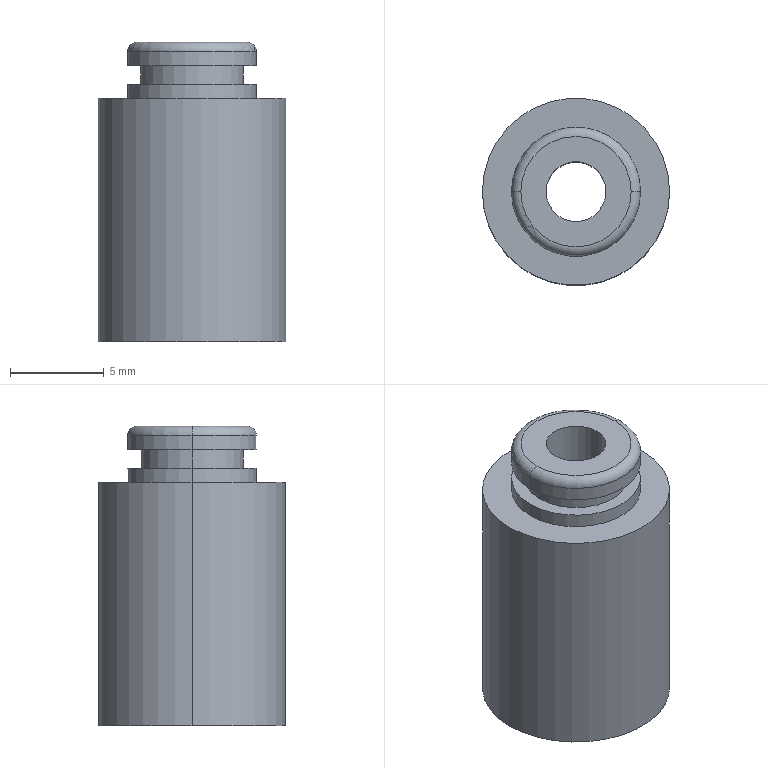Part | STEP file | SS5V1-16S3AD-08B-N1_VV5Q Fittings | 1 solid | 17 faces | box 10 x 10 x 16 mm | volume 989.757 mm3 | cylinder 10 | plane 5 | torus 2 | commonest cylinder face diameters 6.9 x4 3.2 x2 5.5 x2 10 x2
STEP:
#1=CARTESIAN_POINT('',(0.,0.,0.));
#2=DIRECTION('',(0.,0.,1.));
#3=DIRECTION('',(1.,0.,0.));
#4=AXIS2_PLACEMENT_3D('',#1,#2,#3);
#5=CARTESIAN_POINT('',(-3.45,0.,15.5));
#6=VERTEX_POINT('',#5);
#7=CARTESIAN_POINT('',(3.45,0.,15.5));
#8=VERTEX_POINT('',#7);
#9=CARTESIAN_POINT('',(0.,0.,15.5));
#10=DIRECTION('',(0.,0.,-1.));
#11=DIRECTION('',(1.,0.,0.));
#12=AXIS2_PLACEMENT_3D('',#9,#10,#11);
#13=CIRCLE('',#12,3.45);
#14=CARTESIAN_POINT('',(0.,0.,15.5));
#15=DIRECTION('',(0.,0.,1.));
#16=DIRECTION('',(1.,0.,0.));
#17=AXIS2_PLACEMENT_3D('',#14,#15,#16);
#18=TOROIDAL_SURFACE('',#17,2.95,0.5);
#19=CARTESIAN_POINT('',(6.283,0.));
#20=DIRECTION('',(-1.,0.));
#21=VECTOR('',#20,1.);
#22=LINE('',#19,#21);
#23=(GEOMETRIC_REPRESENTATION_CONTEXT(2)PARAMETRIC_REPRESENTATION_CONTEXT()REPRESENTATION_CONTEXT('',''));
#24=DEFINITIONAL_REPRESENTATION('',(#22),#23);
#25=PCURVE('',#18,#24);
#26=CARTESIAN_POINT('',(0.,0.,16.));
#27=DIRECTION('',(0.,0.,-1.));
#28=DIRECTION('',(-1.,0.,0.));
#29=AXIS2_PLACEMENT_3D('',#26,#27,#28);
#30=CYLINDRICAL_SURFACE('',#29,3.45);
#31=CARTESIAN_POINT('',(-3.142,0.5));
#32=DIRECTION('',(1.,0.));
#33=VECTOR('',#32,1.);
#34=LINE('',#31,#33);
#35=(GEOMETRIC_REPRESENTATION_CONTEXT(2)PARAMETRIC_REPRESENTATION_CONTEXT()REPRESENTATION_CONTEXT('',''));
#36=DEFINITIONAL_REPRESENTATION('',(#34),#35);
#37=PCURVE('',#30,#36);
#38=SURFACE_CURVE('',#13,(#25,#37),.PCURVE_S1.);
#39=EDGE_CURVE('',#6,#8,#38,.T.);
#40=ORIENTED_EDGE('',*,*,#39,.F.);
#41=CARTESIAN_POINT('',(-2.95,0.,16.));
#42=VERTEX_POINT('',#41);
#43=CARTESIAN_POINT('',(-2.95,0.,15.5));
#44=DIRECTION('',(0.,1.,0.));
#45=DIRECTION('',(-1.,0.,0.));
#46=AXIS2_PLACEMENT_3D('',#43,#44,#45);
#47=CIRCLE('',#46,0.5);
#48=CARTESIAN_POINT('',(3.142,0.));
#49=DIRECTION('',(0.,1.));
#50=VECTOR('',#49,1.);
#51=LINE('',#48,#50);
#52=(GEOMETRIC_REPRESENTATION_CONTEXT(2)PARAMETRIC_REPRESENTATION_CONTEXT()REPRESENTATION_CONTEXT('',''));
#53=DEFINITIONAL_REPRESENTATION('',(#51),#52);
#54=PCURVE('',#18,#53);
#55=CARTESIAN_POINT('',(0.,0.,15.5));
#56=DIRECTION('',(0.,0.,1.));
#57=DIRECTION('',(1.,0.,0.));
#58=AXIS2_PLACEMENT_3D('',#55,#56,#57);
#59=TOROIDAL_SURFACE('',#58,2.95,0.5);
#60=CARTESIAN_POINT('',(3.142,0.));
#61=DIRECTION('',(0.,1.));
#62=VECTOR('',#61,1.);
#63=LINE('',#60,#62);
#64=(GEOMETRIC_REPRESENTATION_CONTEXT(2)PARAMETRIC_REPRESENTATION_CONTEXT()REPRESENTATION_CONTEXT('',''));
#65=DEFINITIONAL_REPRESENTATION('',(#63),#64);
#66=PCURVE('',#59,#65);
#67=SURFACE_CURVE('',#47,(#54,#66),.PCURVE_S1.);
#68=EDGE_CURVE('',#6,#42,#67,.T.);
#69=ORIENTED_EDGE('',*,*,#68,.T.);
#70=CARTESIAN_POINT('',(2.95,0.,16.));
#71=VERTEX_POINT('',#70);
#72=CARTESIAN_POINT('',(0.,0.,16.));
#73=DIRECTION('',(0.,0.,1.));
#74=DIRECTION('',(1.,0.,0.));
#75=AXIS2_PLACEMENT_3D('',#72,#73,#74);
#76=CIRCLE('',#75,2.95);
#77=CARTESIAN_POINT('',(0.,1.571));
#78=DIRECTION('',(1.,0.));
#79=VECTOR('',#78,1.);
#80=LINE('',#77,#79);
#81=(GEOMETRIC_REPRESENTATION_CONTEXT(2)PARAMETRIC_REPRESENTATION_CONTEXT()REPRESENTATION_CONTEXT('',''));
#82=DEFINITIONAL_REPRESENTATION('',(#80),#81);
#83=PCURVE('',#18,#82);
#84=CARTESIAN_POINT('',(0.,0.,16.));
#85=DIRECTION('',(0.,0.,1.));
#86=DIRECTION('',(1.,0.,0.));
#87=AXIS2_PLACEMENT_3D('',#84,#85,#86);
#88=PLANE('',#87);
#89=CARTESIAN_POINT('',(0.,0.));
#90=DIRECTION('',(1.,0.));
#91=AXIS2_PLACEMENT_2D('',#89,#90);
#92=CIRCLE('',#91,2.95);
#93=(GEOMETRIC_REPRESENTATION_CONTEXT(2)PARAMETRIC_REPRESENTATION_CONTEXT()REPRESENTATION_CONTEXT('',''));
#94=DEFINITIONAL_REPRESENTATION('',(#92),#93);
#95=PCURVE('',#88,#94);
#96=SURFACE_CURVE('',#76,(#83,#95),.PCURVE_S1.);
#97=EDGE_CURVE('',#71,#42,#96,.T.);
#98=ORIENTED_EDGE('',*,*,#97,.F.);
#99=CARTESIAN_POINT('',(2.95,0.,15.5));
#100=DIRECTION('',(0.,-1.,0.));
#101=DIRECTION('',(0.,0.,-1.));
#102=AXIS2_PLACEMENT_3D('',#99,#100,#101);
#103=CIRCLE('',#102,0.5);
#104=CARTESIAN_POINT('',(0.,-1.571));
#105=DIRECTION('',(0.,1.));
#106=VECTOR('',#105,1.);
#107=LINE('',#104,#106);
#108=(GEOMETRIC_REPRESENTATION_CONTEXT(2)PARAMETRIC_REPRESENTATION_CONTEXT()REPRESENTATION_CONTEXT('',''));
#109=DEFINITIONAL_REPRESENTATION('',(#107),#108);
#110=PCURVE('',#18,#109);
#111=CARTESIAN_POINT('',(6.283,-1.571));
#112=DIRECTION('',(0.,1.));
#113=VECTOR('',#112,1.);
#114=LINE('',#111,#113);
#115=(GEOMETRIC_REPRESENTATION_CONTEXT(2)PARAMETRIC_REPRESENTATION_CONTEXT()REPRESENTATION_CONTEXT('',''));
#116=DEFINITIONAL_REPRESENTATION('',(#114),#115);
#117=PCURVE('',#59,#116);
#118=SURFACE_CURVE('',#103,(#110,#117),.PCURVE_S1.);
#119=EDGE_CURVE('',#8,#71,#118,.T.);
#120=ORIENTED_EDGE('',*,*,#119,.F.);
#121=EDGE_LOOP('',(#40,#69,#98,#120));
#122=FACE_BOUND('',#121,.T.);
#123=ADVANCED_FACE('',(#122),#18,.T.);
#124=ORIENTED_EDGE('',*,*,#39,.T.);
#125=CARTESIAN_POINT('',(3.45,0.,14.75));
#126=VERTEX_POINT('',#125);
#127=CARTESIAN_POINT('',(3.45,0.,16.));
#128=DIRECTION('',(0.,0.,-1.));
#129=VECTOR('',#128,1.);
#130=LINE('',#127,#129);
#131=CARTESIAN_POINT('',(3.142,0.));
#132=DIRECTION('',(0.,1.));
#133=VECTOR('',#132,1.);
#134=LINE('',#131,#133);
#135=(GEOMETRIC_REPRESENTATION_CONTEXT(2)PARAMETRIC_REPRESENTATION_CONTEXT()REPRESENTATION_CONTEXT('',''));
#136=DEFINITIONAL_REPRESENTATION('',(#134),#135);
#137=PCURVE('',#30,#136);
#138=CARTESIAN_POINT('',(0.,0.,16.));
#139=DIRECTION('',(0.,0.,-1.));
#140=DIRECTION('',(-1.,0.,0.));
#141=AXIS2_PLACEMENT_3D('',#138,#139,#140);
#142=CYLINDRICAL_SURFACE('',#141,3.45);
#143=CARTESIAN_POINT('',(3.142,0.));
#144=DIRECTION('',(0.,1.));
#145=VECTOR('',#144,1.);
#146=LINE('',#143,#145);
#147=(GEOMETRIC_REPRESENTATION_CONTEXT(2)PARAMETRIC_REPRESENTATION_CONTEXT()REPRESENTATION_CONTEXT('',''));
#148=DEFINITIONAL_REPRESENTATION('',(#146),#147);
#149=PCURVE('',#142,#148);
#150=SURFACE_CURVE('',#130,(#137,#149),.PCURVE_S1.);
#151=EDGE_CURVE('',#8,#126,#150,.T.);
#152=ORIENTED_EDGE('',*,*,#151,.T.);
#153=CARTESIAN_POINT('',(-3.45,0.,14.75));
#154=VERTEX_POINT('',#153);
#155=CARTESIAN_POINT('',(0.,0.,14.75));
#156=DIRECTION('',(0.,0.,1.));
#157=DIRECTION('',(1.,0.,0.));
#158=AXIS2_PLACEMENT_3D('',#155,#156,#157);
#159=CIRCLE('',#158,3.45);
#160=CARTESIAN_POINT('',(3.142,1.25));
#161=DIRECTION('',(-1.,0.));
#162=VECTOR('',#161,1.);
#163=LINE('',#160,#162);
#164=(GEOMETRIC_REPRESENTATION_CONTEXT(2)PARAMETRIC_REPRESENTATION_CONTEXT()REPRESENTATION_CONTEXT('',''));
#165=DEFINITIONAL_REPRESENTATION('',(#163),#164);
#166=PCURVE('',#30,#165);
#167=CARTESIAN_POINT('',(0.,0.,14.75));
#168=DIRECTION('',(0.,0.,1.));
#169=DIRECTION('',(1.,0.,0.));
#170=AXIS2_PLACEMENT_3D('',#167,#168,#169);
#171=PLANE('',#170);
#172=CARTESIAN_POINT('',(0.,0.));
#173=DIRECTION('',(1.,0.));
#174=AXIS2_PLACEMENT_2D('',#172,#173);
#175=CIRCLE('',#174,3.45);
#176=(GEOMETRIC_REPRESENTATION_CONTEXT(2)PARAMETRIC_REPRESENTATION_CONTEXT()REPRESENTATION_CONTEXT('',''));
#177=DEFINITIONAL_REPRESENTATION('',(#175),#176);
#178=PCURVE('',#171,#177);
#179=SURFACE_CURVE('',#159,(#166,#178),.PCURVE_S1.);
#180=EDGE_CURVE('',#126,#154,#179,.T.);
#181=ORIENTED_EDGE('',*,*,#180,.T.);
#182=CARTESIAN_POINT('',(-3.45,0.,16.));
#183=DIRECTION('',(0.,0.,-1.));
#184=VECTOR('',#183,1.);
#185=LINE('',#182,#184);
#186=CARTESIAN_POINT('',(0.,0.));
#187=DIRECTION('',(0.,1.));
#188=VECTOR('',#187,1.);
#189=LINE('',#186,#188);
#190=(GEOMETRIC_REPRESENTATION_CONTEXT(2)PARAMETRIC_REPRESENTATION_CONTEXT()REPRESENTATION_CONTEXT('',''));
#191=DEFINITIONAL_REPRESENTATION('',(#189),#190);
#192=PCURVE('',#30,#191);
#193=CARTESIAN_POINT('',(6.283,0.));
#194=DIRECTION('',(0.,1.));
#195=VECTOR('',#194,1.);
#196=LINE('',#193,#195);
#197=(GEOMETRIC_REPRESENTATION_CONTEXT(2)PARAMETRIC_REPRESENTATION_CONTEXT()REPRESENTATION_CONTEXT('',''));
#198=DEFINITIONAL_REPRESENTATION('',(#196),#197);
#199=PCURVE('',#142,#198);
#200=SURFACE_CURVE('',#185,(#192,#199),.PCURVE_S1.);
#201=EDGE_CURVE('',#6,#154,#200,.T.);
#202=ORIENTED_EDGE('',*,*,#201,.F.);
#203=EDGE_LOOP('',(#124,#152,#181,#202));
#204=FACE_BOUND('',#203,.T.);
#205=ADVANCED_FACE('',(#204),#30,.T.);
#206=CARTESIAN_POINT('',(2.75,0.,14.75));
#207=VERTEX_POINT('',#206);
#208=CARTESIAN_POINT('',(-2.75,0.,14.75));
#209=VERTEX_POINT('',#208);
#210=CARTESIAN_POINT('',(0.,0.,14.75));
#211=DIRECTION('',(0.,0.,1.));
#212=DIRECTION('',(1.,0.,0.));
#213=AXIS2_PLACEMENT_3D('',#210,#211,#212);
#214=CIRCLE('',#213,2.75);
#215=CARTESIAN_POINT('',(0.,0.,14.75));
#216=DIRECTION('',(0.,0.,-1.));
#217=DIRECTION('',(-1.,0.,0.));
#218=AXIS2_PLACEMENT_3D('',#215,#216,#217);
#219=CYLINDRICAL_SURFACE('',#218,2.75);
#220=CARTESIAN_POINT('',(3.142,0.));
#221=DIRECTION('',(-1.,0.));
#222=VECTOR('',#221,1.);
#223=LINE('',#220,#222);
#224=(GEOMETRIC_REPRESENTATION_CONTEXT(2)PARAMETRIC_REPRESENTATION_CONTEXT()REPRESENTATION_CONTEXT('',''));
#225=DEFINITIONAL_REPRESENTATION('',(#223),#224);
#226=PCURVE('',#219,#225);
#227=CARTESIAN_POINT('',(0.,0.));
#228=DIRECTION('',(1.,0.));
#229=AXIS2_PLACEMENT_2D('',#227,#228);
#230=CIRCLE('',#229,2.75);
#231=(GEOMETRIC_REPRESENTATION_CONTEXT(2)PARAMETRIC_REPRESENTATION_CONTEXT()REPRESENTATION_CONTEXT('',''));
#232=DEFINITIONAL_REPRESENTATION('',(#230),#231);
#233=PCURVE('',#171,#232);
#234=SURFACE_CURVE('',#214,(#226,#233),.PCURVE_S1.);
#235=EDGE_CURVE('',#207,#209,#234,.T.);
#236=ORIENTED_EDGE('',*,*,#235,.F.);
#237=CARTESIAN_POINT('',(2.75,0.,13.75));
#238=VERTEX_POINT('',#237);
#239=CARTESIAN_POINT('',(2.75,0.,14.75));
#240=DIRECTION('',(0.,0.,-1.));
#241=VECTOR('',#240,1.);
#242=LINE('',#239,#241);
#243=CARTESIAN_POINT('',(3.142,0.));
#244=DIRECTION('',(0.,1.));
#245=VECTOR('',#244,1.);
#246=LINE('',#243,#245);
#247=(GEOMETRIC_REPRESENTATION_CONTEXT(2)PARAMETRIC_REPRESENTATION_CONTEXT()REPRESENTATION_CONTEXT('',''));
#248=DEFINITIONAL_REPRESENTATION('',(#246),#247);
#249=PCURVE('',#219,#248);
#250=CARTESIAN_POINT('',(0.,0.,14.75));
#251=DIRECTION('',(0.,0.,-1.));
#252=DIRECTION('',(-1.,0.,0.));
#253=AXIS2_PLACEMENT_3D('',#250,#251,#252);
#254=CYLINDRICAL_SURFACE('',#253,2.75);
#255=CARTESIAN_POINT('',(3.142,0.));
#256=DIRECTION('',(0.,1.));
#257=VECTOR('',#256,1.);
#258=LINE('',#255,#257);
#259=(GEOMETRIC_REPRESENTATION_CONTEXT(2)PARAMETRIC_REPRESENTATION_CONTEXT()REPRESENTATION_CONTEXT('',''));
#260=DEFINITIONAL_REPRESENTATION('',(#258),#259);
#261=PCURVE('',#254,#260);
#262=SURFACE_CURVE('',#242,(#249,#261),.PCURVE_S1.);
#263=EDGE_CURVE('',#207,#238,#262,.T.);
#264=ORIENTED_EDGE('',*,*,#263,.T.);
#265=CARTESIAN_POINT('',(-2.75,0.,13.75));
#266=VERTEX_POINT('',#265);
#267=CARTESIAN_POINT('',(0.,0.,13.75));
#268=DIRECTION('',(0.,0.,1.));
#269=DIRECTION('',(1.,0.,0.));
#270=AXIS2_PLACEMENT_3D('',#267,#268,#269);
#271=CIRCLE('',#270,2.75);
#272=CARTESIAN_POINT('',(3.142,1.));
#273=DIRECTION('',(-1.,0.));
#274=VECTOR('',#273,1.);
#275=LINE('',#272,#274);
#276=(GEOMETRIC_REPRESENTATION_CONTEXT(2)PARAMETRIC_REPRESENTATION_CONTEXT()REPRESENTATION_CONTEXT('',''));
#277=DEFINITIONAL_REPRESENTATION('',(#275),#276);
#278=PCURVE('',#219,#277);
#279=CARTESIAN_POINT('',(0.,0.,13.75));
#280=DIRECTION('',(0.,0.,1.));
#281=DIRECTION('',(1.,0.,0.));
#282=AXIS2_PLACEMENT_3D('',#279,#280,#281);
#283=PLANE('',#282);
#284=CARTESIAN_POINT('',(0.,0.));
#285=DIRECTION('',(1.,0.));
#286=AXIS2_PLACEMENT_2D('',#284,#285);
#287=CIRCLE('',#286,2.75);
#288=(GEOMETRIC_REPRESENTATION_CONTEXT(2)PARAMETRIC_REPRESENTATION_CONTEXT()REPRESENTATION_CONTEXT('',''));
#289=DEFINITIONAL_REPRESENTATION('',(#287),#288);
#290=PCURVE('',#283,#289);
#291=SURFACE_CURVE('',#271,(#278,#290),.PCURVE_S1.);
#292=EDGE_CURVE('',#238,#266,#291,.T.);
#293=ORIENTED_EDGE('',*,*,#292,.T.);
#294=CARTESIAN_POINT('',(-2.75,0.,14.75));
#295=DIRECTION('',(0.,0.,-1.));
#296=VECTOR('',#295,1.);
#297=LINE('',#294,#296);
#298=CARTESIAN_POINT('',(0.,0.));
#299=DIRECTION('',(0.,1.));
#300=VECTOR('',#299,1.);
#301=LINE('',#298,#300);
#302=(GEOMETRIC_REPRESENTATION_CONTEXT(2)PARAMETRIC_REPRESENTATION_CONTEXT()REPRESENTATION_CONTEXT('',''));
#303=DEFINITIONAL_REPRESENTATION('',(#301),#302);
#304=PCURVE('',#219,#303);
#305=CARTESIAN_POINT('',(6.283,0.));
#306=DIRECTION('',(0.,1.));
#307=VECTOR('',#306,1.);
#308=LINE('',#305,#307);
#309=(GEOMETRIC_REPRESENTATION_CONTEXT(2)PARAMETRIC_REPRESENTATION_CONTEXT()REPRESENTATION_CONTEXT('',''));
#310=DEFINITIONAL_REPRESENTATION('',(#308),#309);
#311=PCURVE('',#254,#310);
#312=SURFACE_CURVE('',#297,(#304,#311),.PCURVE_S1.);
#313=EDGE_CURVE('',#209,#266,#312,.T.);
#314=ORIENTED_EDGE('',*,*,#313,.F.);
#315=EDGE_LOOP('',(#236,#264,#293,#314));
#316=FACE_BOUND('',#315,.T.);
#317=ADVANCED_FACE('',(#316),#219,.T.);
#318=CARTESIAN_POINT('',(3.45,0.,13.75));
#319=VERTEX_POINT('',#318);
#320=CARTESIAN_POINT('',(-3.45,0.,13.75));
#321=VERTEX_POINT('',#320);
#322=CARTESIAN_POINT('',(0.,0.,13.75));
#323=DIRECTION('',(0.,0.,1.));
#324=DIRECTION('',(1.,0.,0.));
#325=AXIS2_PLACEMENT_3D('',#322,#323,#324);
#326=CIRCLE('',#325,3.45);
#327=CARTESIAN_POINT('',(0.,0.,13.75));
#328=DIRECTION('',(0.,0.,-1.));
#329=DIRECTION('',(-1.,0.,0.));
#330=AXIS2_PLACEMENT_3D('',#327,#328,#329);
#331=CYLINDRICAL_SURFACE('',#330,3.45);
#332=CARTESIAN_POINT('',(3.142,0.));
#333=DIRECTION('',(-1.,0.));
#334=VECTOR('',#333,1.);
#335=LINE('',#332,#334);
#336=(GEOMETRIC_REPRESENTATION_CONTEXT(2)PARAMETRIC_REPRESENTATION_CONTEXT()REPRESENTATION_CONTEXT('',''));
#337=DEFINITIONAL_REPRESENTATION('',(#335),#336);
#338=PCURVE('',#331,#337);
#339=CARTESIAN_POINT('',(0.,0.));
#340=DIRECTION('',(1.,0.));
#341=AXIS2_PLACEMENT_2D('',#339,#340);
#342=CIRCLE('',#341,3.45);
#343=(GEOMETRIC_REPRESENTATION_CONTEXT(2)PARAMETRIC_REPRESENTATION_CONTEXT()REPRESENTATION_CONTEXT('',''));
#344=DEFINITIONAL_REPRESENTATION('',(#342),#343);
#345=PCURVE('',#283,#344);
#346=SURFACE_CURVE('',#326,(#338,#345),.PCURVE_S1.);
#347=EDGE_CURVE('',#319,#321,#346,.T.);
#348=ORIENTED_EDGE('',*,*,#347,.F.);
#349=CARTESIAN_POINT('',(3.45,0.,13.));
#350=VERTEX_POINT('',#349);
#351=CARTESIAN_POINT('',(3.45,0.,13.75));
#352=DIRECTION('',(0.,0.,-1.));
#353=VECTOR('',#352,1.);
#354=LINE('',#351,#353);
#355=CARTESIAN_POINT('',(3.142,0.));
#356=DIRECTION('',(0.,1.));
#357=VECTOR('',#356,1.);
#358=LINE('',#355,#357);
#359=(GEOMETRIC_REPRESENTATION_CONTEXT(2)PARAMETRIC_REPRESENTATION_CONTEXT()REPRESENTATION_CONTEXT('',''));
#360=DEFINITIONAL_REPRESENTATION('',(#358),#359);
#361=PCURVE('',#331,#360);
#362=CARTESIAN_POINT('',(0.,0.,13.75));
#363=DIRECTION('',(0.,0.,-1.));
#364=DIRECTION('',(-1.,0.,0.));
#365=AXIS2_PLACEMENT_3D('',#362,#363,#364);
#366=CYLINDRICAL_SURFACE('',#365,3.45);
#367=CARTESIAN_POINT('',(3.142,0.));
#368=DIRECTION('',(0.,1.));
#369=VECTOR('',#368,1.);
#370=LINE('',#367,#369);
#371=(GEOMETRIC_REPRESENTATION_CONTEXT(2)PARAMETRIC_REPRESENTATION_CONTEXT()REPRESENTATION_CONTEXT('',''));
#372=DEFINITIONAL_REPRESENTATION('',(#370),#371);
#373=PCURVE('',#366,#372);
#374=SURFACE_CURVE('',#354,(#361,#373),.PCURVE_S1.);
#375=EDGE_CURVE('',#319,#350,#374,.T.);
#376=ORIENTED_EDGE('',*,*,#375,.T.);
#377=CARTESIAN_POINT('',(-3.45,0.,13.));
#378=VERTEX_POINT('',#377);
#379=CARTESIAN_POINT('',(0.,0.,13.));
#380=DIRECTION('',(0.,0.,1.));
#381=DIRECTION('',(1.,0.,0.));
#382=AXIS2_PLACEMENT_3D('',#379,#380,#381);
#383=CIRCLE('',#382,3.45);
#384=CARTESIAN_POINT('',(3.142,0.75));
#385=DIRECTION('',(-1.,0.));
#386=VECTOR('',#385,1.);
#387=LINE('',#384,#386);
#388=(GEOMETRIC_REPRESENTATION_CONTEXT(2)PARAMETRIC_REPRESENTATION_CONTEXT()REPRESENTATION_CONTEXT('',''));
#389=DEFINITIONAL_REPRESENTATION('',(#387),#388);
#390=PCURVE('',#331,#389);
#391=CARTESIAN_POINT('',(0.,0.,13.));
#392=DIRECTION('',(0.,0.,1.));
#393=DIRECTION('',(1.,0.,0.));
#394=AXIS2_PLACEMENT_3D('',#391,#392,#393);
#395=PLANE('',#394);
#396=CARTESIAN_POINT('',(0.,0.));
#397=DIRECTION('',(1.,0.));
#398=AXIS2_PLACEMENT_2D('',#396,#397);
#399=CIRCLE('',#398,3.45);
#400=(GEOMETRIC_REPRESENTATION_CONTEXT(2)PARAMETRIC_REPRESENTATION_CONTEXT()REPRESENTATION_CONTEXT('',''));
#401=DEFINITIONAL_REPRESENTATION('',(#399),#400);
#402=PCURVE('',#395,#401);
#403=SURFACE_CURVE('',#383,(#390,#402),.PCURVE_S1.);
#404=EDGE_CURVE('',#350,#378,#403,.T.);
#405=ORIENTED_EDGE('',*,*,#404,.T.);
#406=CARTESIAN_POINT('',(-3.45,0.,13.75));
#407=DIRECTION('',(0.,0.,-1.));
#408=VECTOR('',#407,1.);
#409=LINE('',#406,#408);
#410=CARTESIAN_POINT('',(0.,0.));
#411=DIRECTION('',(0.,1.));
#412=VECTOR('',#411,1.);
#413=LINE('',#410,#412);
#414=(GEOMETRIC_REPRESENTATION_CONTEXT(2)PARAMETRIC_REPRESENTATION_CONTEXT()REPRESENTATION_CONTEXT('',''));
#415=DEFINITIONAL_REPRESENTATION('',(#413),#414);
#416=PCURVE('',#331,#415);
#417=CARTESIAN_POINT('',(6.283,0.));
#418=DIRECTION('',(0.,1.));
#419=VECTOR('',#418,1.);
#420=LINE('',#417,#419);
#421=(GEOMETRIC_REPRESENTATION_CONTEXT(2)PARAMETRIC_REPRESENTATION_CONTEXT()REPRESENTATION_CONTEXT('',''));
#422=DEFINITIONAL_REPRESENTATION('',(#420),#421);
#423=PCURVE('',#366,#422);
#424=SURFACE_CURVE('',#409,(#416,#423),.PCURVE_S1.);
#425=EDGE_CURVE('',#321,#378,#424,.T.);
#426=ORIENTED_EDGE('',*,*,#425,.F.);
#427=EDGE_LOOP('',(#348,#376,#405,#426));
#428=FACE_BOUND('',#427,.T.);
#429=ADVANCED_FACE('',(#428),#331,.T.);
#430=CARTESIAN_POINT('',(-1.6,0.,16.));
#431=VERTEX_POINT('',#430);
#432=CARTESIAN_POINT('',(-1.6,0.,0.));
#433=VERTEX_POINT('',#432);
#434=CARTESIAN_POINT('',(-1.6,0.,13.));
#435=DIRECTION('',(0.,0.,-1.));
#436=VECTOR('',#435,1.);
#437=LINE('',#434,#436);
#438=CARTESIAN_POINT('',(0.,0.,13.));
#439=DIRECTION('',(0.,0.,-1.));
#440=DIRECTION('',(-1.,0.,0.));
#441=AXIS2_PLACEMENT_3D('',#438,#439,#440);
#442=CYLINDRICAL_SURFACE('',#441,1.6);
#443=CARTESIAN_POINT('',(6.283,0.));
#444=DIRECTION('',(0.,1.));
#445=VECTOR('',#444,1.);
#446=LINE('',#443,#445);
#447=(GEOMETRIC_REPRESENTATION_CONTEXT(2)PARAMETRIC_REPRESENTATION_CONTEXT()REPRESENTATION_CONTEXT('',''));
#448=DEFINITIONAL_REPRESENTATION('',(#446),#447);
#449=PCURVE('',#442,#448);
#450=CARTESIAN_POINT('',(0.,0.,13.));
#451=DIRECTION('',(0.,0.,-1.));
#452=DIRECTION('',(-1.,0.,0.));
#453=AXIS2_PLACEMENT_3D('',#450,#451,#452);
#454=CYLINDRICAL_SURFACE('',#453,1.6);
#455=CARTESIAN_POINT('',(0.,0.));
#456=DIRECTION('',(0.,1.));
#457=VECTOR('',#456,1.);
#458=LINE('',#455,#457);
#459=(GEOMETRIC_REPRESENTATION_CONTEXT(2)PARAMETRIC_REPRESENTATION_CONTEXT()REPRESENTATION_CONTEXT('',''));
#460=DEFINITIONAL_REPRESENTATION('',(#458),#459);
#461=PCURVE('',#454,#460);
#462=SURFACE_CURVE('',#437,(#449,#461),.PCURVE_S1.);
#463=EDGE_CURVE('',#431,#433,#462,.T.);
#464=ORIENTED_EDGE('',*,*,#463,.T.);
#465=CARTESIAN_POINT('',(1.6,0.,0.));
#466=VERTEX_POINT('',#465);
#467=CARTESIAN_POINT('',(0.,0.,0.));
#468=DIRECTION('',(0.,0.,1.));
#469=DIRECTION('',(1.,0.,0.));
#470=AXIS2_PLACEMENT_3D('',#467,#468,#469);
#471=CIRCLE('',#470,1.6);
#472=CARTESIAN_POINT('',(9.425,13.));
#473=DIRECTION('',(-1.,0.));
#474=VECTOR('',#473,1.);
#475=LINE('',#472,#474);
#476=(GEOMETRIC_REPRESENTATION_CONTEXT(2)PARAMETRIC_REPRESENTATION_CONTEXT()REPRESENTATION_CONTEXT('',''));
#477=DEFINITIONAL_REPRESENTATION('',(#475),#476);
#478=PCURVE('',#442,#477);
#479=CARTESIAN_POINT('',(0.,0.,0.));
#480=DIRECTION('',(0.,0.,1.));
#481=DIRECTION('',(1.,0.,0.));
#482=AXIS2_PLACEMENT_3D('',#479,#480,#481);
#483=PLANE('',#482);
#484=CARTESIAN_POINT('',(0.,0.));
#485=DIRECTION('',(1.,0.));
#486=AXIS2_PLACEMENT_2D('',#484,#485);
#487=CIRCLE('',#486,1.6);
#488=(GEOMETRIC_REPRESENTATION_CONTEXT(2)PARAMETRIC_REPRESENTATION_CONTEXT()REPRESENTATION_CONTEXT('',''));
#489=DEFINITIONAL_REPRESENTATION('',(#487),#488);
#490=PCURVE('',#483,#489);
#491=SURFACE_CURVE('',#471,(#478,#490),.PCURVE_S1.);
#492=EDGE_CURVE('',#433,#466,#491,.T.);
#493=ORIENTED_EDGE('',*,*,#492,.T.);
#494=CARTESIAN_POINT('',(1.6,0.,16.));
#495=VERTEX_POINT('',#494);
#496=CARTESIAN_POINT('',(1.6,0.,13.));
#497=DIRECTION('',(0.,0.,-1.));
#498=VECTOR('',#497,1.);
#499=LINE('',#496,#498);
#500=CARTESIAN_POINT('',(3.142,0.));
#501=DIRECTION('',(0.,1.));
#502=VECTOR('',#501,1.);
#503=LINE('',#500,#502);
#504=(GEOMETRIC_REPRESENTATION_CONTEXT(2)PARAMETRIC_REPRESENTATION_CONTEXT()REPRESENTATION_CONTEXT('',''));
#505=DEFINITIONAL_REPRESENTATION('',(#503),#504);
#506=PCURVE('',#442,#505);
#507=CARTESIAN_POINT('',(3.142,0.));
#508=DIRECTION('',(0.,1.));
#509=VECTOR('',#508,1.);
#510=LINE('',#507,#509);
#511=(GEOMETRIC_REPRESENTATION_CONTEXT(2)PARAMETRIC_REPRESENTATION_CONTEXT()REPRESENTATION_CONTEXT('',''));
#512=DEFINITIONAL_REPRESENTATION('',(#510),#511);
#513=PCURVE('',#454,#512);
#514=SURFACE_CURVE('',#499,(#506,#513),.PCURVE_S1.);
#515=EDGE_CURVE('',#495,#466,#514,.T.);
#516=ORIENTED_EDGE('',*,*,#515,.F.);
#517=CARTESIAN_POINT('',(0.,0.,16.));
#518=DIRECTION('',(0.,0.,1.));
#519=DIRECTION('',(1.,0.,0.));
#520=AXIS2_PLACEMENT_3D('',#517,#518,#519);
#521=CIRCLE('',#520,1.6);
#522=CARTESIAN_POINT('',(9.425,-3.));
#523=DIRECTION('',(-1.,0.));
#524=VECTOR('',#523,1.);
#525=LINE('',#522,#524);
#526=(GEOMETRIC_REPRESENTATION_CONTEXT(2)PARAMETRIC_REPRESENTATION_CONTEXT()REPRESENTATION_CONTEXT('',''));
#527=DEFINITIONAL_REPRESENTATION('',(#525),#526);
#528=PCURVE('',#442,#527);
#529=CARTESIAN_POINT('',(0.,0.));
#530=DIRECTION('',(1.,0.));
#531=AXIS2_PLACEMENT_2D('',#529,#530);
#532=CIRCLE('',#531,1.6);
#533=(GEOMETRIC_REPRESENTATION_CONTEXT(2)PARAMETRIC_REPRESENTATION_CONTEXT()REPRESENTATION_CONTEXT('',''));
#534=DEFINITIONAL_REPRESENTATION('',(#532),#533);
#535=PCURVE('',#88,#534);
#536=SURFACE_CURVE('',#521,(#528,#535),.PCURVE_S1.);
#537=EDGE_CURVE('',#431,#495,#536,.T.);
#538=ORIENTED_EDGE('',*,*,#537,.F.);
#539=EDGE_LOOP('',(#464,#493,#516,#538));
#540=FACE_BOUND('',#539,.F.);
#541=ADVANCED_FACE('',(#540),#442,.F.);
#542=CARTESIAN_POINT('',(5.,0.,13.));
#543=VERTEX_POINT('',#542);
#544=CARTESIAN_POINT('',(-5.,0.,13.));
#545=VERTEX_POINT('',#544);
#546=CARTESIAN_POINT('',(0.,0.,13.));
#547=DIRECTION('',(0.,0.,1.));
#548=DIRECTION('',(1.,0.,0.));
#549=AXIS2_PLACEMENT_3D('',#546,#547,#548);
#550=CIRCLE('',#549,5.);
#551=CARTESIAN_POINT('',(0.,0.,13.));
#552=DIRECTION('',(0.,0.,-1.));
#553=DIRECTION('',(-1.,0.,0.));
#554=AXIS2_PLACEMENT_3D('',#551,#552,#553);
#555=CYLINDRICAL_SURFACE('',#554,5.);
#556=CARTESIAN_POINT('',(3.142,0.));
#557=DIRECTION('',(-1.,0.));
#558=VECTOR('',#557,1.);
#559=LINE('',#556,#558);
#560=(GEOMETRIC_REPRESENTATION_CONTEXT(2)PARAMETRIC_REPRESENTATION_CONTEXT()REPRESENTATION_CONTEXT('',''));
#561=DEFINITIONAL_REPRESENTATION('',(#559),#560);
#562=PCURVE('',#555,#561);
#563=CARTESIAN_POINT('',(0.,0.));
#564=DIRECTION('',(1.,0.));
#565=AXIS2_PLACEMENT_2D('',#563,#564);
#566=CIRCLE('',#565,5.);
#567=(GEOMETRIC_REPRESENTATION_CONTEXT(2)PARAMETRIC_REPRESENTATION_CONTEXT()REPRESENTATION_CONTEXT('',''));
#568=DEFINITIONAL_REPRESENTATION('',(#566),#567);
#569=PCURVE('',#395,#568);
#570=SURFACE_CURVE('',#550,(#562,#569),.PCURVE_S1.);
#571=EDGE_CURVE('',#543,#545,#570,.T.);
#572=ORIENTED_EDGE('',*,*,#571,.F.);
#573=CARTESIAN_POINT('',(5.,0.,0.));
#574=VERTEX_POINT('',#573);
#575=CARTESIAN_POINT('',(5.,0.,13.));
#576=DIRECTION('',(0.,0.,-1.));
#577=VECTOR('',#576,1.);
#578=LINE('',#575,#577);
#579=CARTESIAN_POINT('',(3.142,0.));
#580=DIRECTION('',(0.,1.));
#581=VECTOR('',#580,1.);
#582=LINE('',#579,#581);
#583=(GEOMETRIC_REPRESENTATION_CONTEXT(2)PARAMETRIC_REPRESENTATION_CONTEXT()REPRESENTATION_CONTEXT('',''));
#584=DEFINITIONAL_REPRESENTATION('',(#582),#583);
#585=PCURVE('',#555,#584);
#586=CARTESIAN_POINT('',(0.,0.,13.));
#587=DIRECTION('',(0.,0.,-1.));
#588=DIRECTION('',(-1.,0.,0.));
#589=AXIS2_PLACEMENT_3D('',#586,#587,#588);
#590=CYLINDRICAL_SURFACE('',#589,5.);
#591=CARTESIAN_POINT('',(3.142,0.));
#592=DIRECTION('',(0.,1.));
#593=VECTOR('',#592,1.);
#594=LINE('',#591,#593);
#595=(GEOMETRIC_REPRESENTATION_CONTEXT(2)PARAMETRIC_REPRESENTATION_CONTEXT()REPRESENTATION_CONTEXT('',''));
#596=DEFINITIONAL_REPRESENTATION('',(#594),#595);
#597=PCURVE('',#590,#596);
#598=SURFACE_CURVE('',#578,(#585,#597),.PCURVE_S1.);
#599=EDGE_CURVE('',#543,#574,#598,.T.);
#600=ORIENTED_EDGE('',*,*,#599,.T.);
#601=CARTESIAN_POINT('',(-5.,0.,0.));
#602=VERTEX_POINT('',#601);
#603=CARTESIAN_POINT('',(0.,0.,0.));
#604=DIRECTION('',(0.,0.,1.));
#605=DIRECTION('',(1.,0.,0.));
#606=AXIS2_PLACEMENT_3D('',#603,#604,#605);
#607=CIRCLE('',#606,5.);
#608=CARTESIAN_POINT('',(3.142,13.));
#609=DIRECTION('',(-1.,0.));
#610=VECTOR('',#609,1.);
#611=LINE('',#608,#610);
#612=(GEOMETRIC_REPRESENTATION_CONTEXT(2)PARAMETRIC_REPRESENTATION_CONTEXT()REPRESENTATION_CONTEXT('',''));
#613=DEFINITIONAL_REPRESENTATION('',(#611),#612);
#614=PCURVE('',#555,#613);
#615=CARTESIAN_POINT('',(0.,0.));
#616=DIRECTION('',(1.,0.));
#617=AXIS2_PLACEMENT_2D('',#615,#616);
#618=CIRCLE('',#617,5.);
#619=(GEOMETRIC_REPRESENTATION_CONTEXT(2)PARAMETRIC_REPRESENTATION_CONTEXT()REPRESENTATION_CONTEXT('',''));
#620=DEFINITIONAL_REPRESENTATION('',(#618),#619);
#621=PCURVE('',#483,#620);
#622=SURFACE_CURVE('',#607,(#614,#621),.PCURVE_S1.);
#623=EDGE_CURVE('',#574,#602,#622,.T.);
#624=ORIENTED_EDGE('',*,*,#623,.T.);
#625=CARTESIAN_POINT('',(-5.,0.,13.));
#626=DIRECTION('',(0.,0.,-1.));
#627=VECTOR('',#626,1.);
#628=LINE('',#625,#627);
#629=CARTESIAN_POINT('',(0.,0.));
#630=DIRECTION('',(0.,1.));
#631=VECTOR('',#630,1.);
#632=LINE('',#629,#631);
#633=(GEOMETRIC_REPRESENTATION_CONTEXT(2)PARAMETRIC_REPRESENTATION_CONTEXT()REPRESENTATION_CONTEXT('',''));
#634=DEFINITIONAL_REPRESENTATION('',(#632),#633);
#635=PCURVE('',#555,#634);
#636=CARTESIAN_POINT('',(6.283,0.));
#637=DIRECTION('',(0.,1.));
#638=VECTOR('',#637,1.);
#639=LINE('',#636,#638);
#640=(GEOMETRIC_REPRESENTATION_CONTEXT(2)PARAMETRIC_REPRESENTATION_CONTEXT()REPRESENTATION_CONTEXT('',''));
#641=DEFINITIONAL_REPRESENTATION('',(#639),#640);
#642=PCURVE('',#590,#641);
#643=SURFACE_CURVE('',#628,(#635,#642),.PCURVE_S1.);
#644=EDGE_CURVE('',#545,#602,#643,.T.);
#645=ORIENTED_EDGE('',*,*,#644,.F.);
#646=EDGE_LOOP('',(#572,#600,#624,#645));
#647=FACE_BOUND('',#646,.T.);
#648=ADVANCED_FACE('',(#647),#555,.T.);
#649=CARTESIAN_POINT('',(0.,0.,13.75));
#650=DIRECTION('',(0.,0.,1.));
#651=DIRECTION('',(1.,0.,0.));
#652=AXIS2_PLACEMENT_3D('',#649,#650,#651);
#653=CIRCLE('',#652,3.45);
#654=CARTESIAN_POINT('',(0.,0.));
#655=DIRECTION('',(1.,0.));
#656=AXIS2_PLACEMENT_2D('',#654,#655);
#657=CIRCLE('',#656,3.45);
#658=(GEOMETRIC_REPRESENTATION_CONTEXT(2)PARAMETRIC_REPRESENTATION_CONTEXT()REPRESENTATION_CONTEXT('',''));
#659=DEFINITIONAL_REPRESENTATION('',(#657),#658);
#660=PCURVE('',#283,#659);
#661=CARTESIAN_POINT('',(9.425,0.));
#662=DIRECTION('',(-1.,0.));
#663=VECTOR('',#662,1.);
#664=LINE('',#661,#663);
#665=(GEOMETRIC_REPRESENTATION_CONTEXT(2)PARAMETRIC_REPRESENTATION_CONTEXT()REPRESENTATION_CONTEXT('',''));
#666=DEFINITIONAL_REPRESENTATION('',(#664),#665);
#667=PCURVE('',#366,#666);
#668=SURFACE_CURVE('',#653,(#660,#667),.PCURVE_S1.);
#669=EDGE_CURVE('',#321,#319,#668,.T.);
#670=ORIENTED_EDGE('',*,*,#669,.T.);
#671=ORIENTED_EDGE('',*,*,#347,.T.);
#672=EDGE_LOOP('',(#670,#671));
#673=FACE_BOUND('',#672,.T.);
#674=CARTESIAN_POINT('',(0.,0.,13.75));
#675=DIRECTION('',(0.,0.,1.));
#676=DIRECTION('',(1.,0.,0.));
#677=AXIS2_PLACEMENT_3D('',#674,#675,#676);
#678=CIRCLE('',#677,2.75);
#679=CARTESIAN_POINT('',(0.,0.));
#680=DIRECTION('',(1.,0.));
#681=AXIS2_PLACEMENT_2D('',#679,#680);
#682=CIRCLE('',#681,2.75);
#683=(GEOMETRIC_REPRESENTATION_CONTEXT(2)PARAMETRIC_REPRESENTATION_CONTEXT()REPRESENTATION_CONTEXT('',''));
#684=DEFINITIONAL_REPRESENTATION('',(#682),#683);
#685=PCURVE('',#283,#684);
#686=CARTESIAN_POINT('',(9.425,1.));
#687=DIRECTION('',(-1.,0.));
#688=VECTOR('',#687,1.);
#689=LINE('',#686,#688);
#690=(GEOMETRIC_REPRESENTATION_CONTEXT(2)PARAMETRIC_REPRESENTATION_CONTEXT()REPRESENTATION_CONTEXT('',''));
#691=DEFINITIONAL_REPRESENTATION('',(#689),#690);
#692=PCURVE('',#254,#691);
#693=SURFACE_CURVE('',#678,(#685,#692),.PCURVE_S1.);
#694=EDGE_CURVE('',#266,#238,#693,.T.);
#695=ORIENTED_EDGE('',*,*,#694,.F.);
#696=ORIENTED_EDGE('',*,*,#292,.F.);
#697=EDGE_LOOP('',(#695,#696));
#698=FACE_BOUND('',#697,.T.);
#699=ADVANCED_FACE('',(#673,#698),#283,.T.);
#700=CARTESIAN_POINT('',(0.,0.,13.));
#701=DIRECTION('',(0.,0.,1.));
#702=DIRECTION('',(1.,0.,0.));
#703=AXIS2_PLACEMENT_3D('',#700,#701,#702);
#704=CIRCLE('',#703,5.);
#705=CARTESIAN_POINT('',(0.,0.));
#706=DIRECTION('',(1.,0.));
#707=AXIS2_PLACEMENT_2D('',#705,#706);
#708=CIRCLE('',#707,5.);
#709=(GEOMETRIC_REPRESENTATION_CONTEXT(2)PARAMETRIC_REPRESENTATION_CONTEXT()REPRESENTATION_CONTEXT('',''));
#710=DEFINITIONAL_REPRESENTATION('',(#708),#709);
#711=PCURVE('',#395,#710);
#712=CARTESIAN_POINT('',(9.425,0.));
#713=DIRECTION('',(-1.,0.));
#714=VECTOR('',#713,1.);
#715=LINE('',#712,#714);
#716=(GEOMETRIC_REPRESENTATION_CONTEXT(2)PARAMETRIC_REPRESENTATION_CONTEXT()REPRESENTATION_CONTEXT('',''));
#717=DEFINITIONAL_REPRESENTATION('',(#715),#716);
#718=PCURVE('',#590,#717);
#719=SURFACE_CURVE('',#704,(#711,#718),.PCURVE_S1.);
#720=EDGE_CURVE('',#545,#543,#719,.T.);
#721=ORIENTED_EDGE('',*,*,#720,.T.);
#722=ORIENTED_EDGE('',*,*,#571,.T.);
#723=EDGE_LOOP('',(#721,#722));
#724=FACE_BOUND('',#723,.T.);
#725=CARTESIAN_POINT('',(0.,0.,13.));
#726=DIRECTION('',(0.,0.,1.));
#727=DIRECTION('',(1.,0.,0.));
#728=AXIS2_PLACEMENT_3D('',#725,#726,#727);
#729=CIRCLE('',#728,3.45);
#730=CARTESIAN_POINT('',(0.,0.));
#731=DIRECTION('',(1.,0.));
#732=AXIS2_PLACEMENT_2D('',#730,#731);
#733=CIRCLE('',#732,3.45);
#734=(GEOMETRIC_REPRESENTATION_CONTEXT(2)PARAMETRIC_REPRESENTATION_CONTEXT()REPRESENTATION_CONTEXT('',''));
#735=DEFINITIONAL_REPRESENTATION('',(#733),#734);
#736=PCURVE('',#395,#735);
#737=CARTESIAN_POINT('',(9.425,0.75));
#738=DIRECTION('',(-1.,0.));
#739=VECTOR('',#738,1.);
#740=LINE('',#737,#739);
#741=(GEOMETRIC_REPRESENTATION_CONTEXT(2)PARAMETRIC_REPRESENTATION_CONTEXT()REPRESENTATION_CONTEXT('',''));
#742=DEFINITIONAL_REPRESENTATION('',(#740),#741);
#743=PCURVE('',#366,#742);
#744=SURFACE_CURVE('',#729,(#736,#743),.PCURVE_S1.);
#745=EDGE_CURVE('',#378,#350,#744,.T.);
#746=ORIENTED_EDGE('',*,*,#745,.F.);
#747=ORIENTED_EDGE('',*,*,#404,.F.);
#748=EDGE_LOOP('',(#746,#747));
#749=FACE_BOUND('',#748,.T.);
#750=ADVANCED_FACE('',(#724,#749),#395,.T.);
#751=CARTESIAN_POINT('',(0.,0.,0.));
#752=DIRECTION('',(0.,0.,1.));
#753=DIRECTION('',(1.,0.,0.));
#754=AXIS2_PLACEMENT_3D('',#751,#752,#753);
#755=CIRCLE('',#754,5.);
#756=CARTESIAN_POINT('',(0.,0.));
#757=DIRECTION('',(1.,0.));
#758=AXIS2_PLACEMENT_2D('',#756,#757);
#759=CIRCLE('',#758,5.);
#760=(GEOMETRIC_REPRESENTATION_CONTEXT(2)PARAMETRIC_REPRESENTATION_CONTEXT()REPRESENTATION_CONTEXT('',''));
#761=DEFINITIONAL_REPRESENTATION('',(#759),#760);
#762=PCURVE('',#483,#761);
#763=CARTESIAN_POINT('',(9.425,13.));
#764=DIRECTION('',(-1.,0.));
#765=VECTOR('',#764,1.);
#766=LINE('',#763,#765);
#767=(GEOMETRIC_REPRESENTATION_CONTEXT(2)PARAMETRIC_REPRESENTATION_CONTEXT()REPRESENTATION_CONTEXT('',''));
#768=DEFINITIONAL_REPRESENTATION('',(#766),#767);
#769=PCURVE('',#590,#768);
#770=SURFACE_CURVE('',#755,(#762,#769),.PCURVE_S1.);
#771=EDGE_CURVE('',#602,#574,#770,.T.);
#772=ORIENTED_EDGE('',*,*,#771,.F.);
#773=ORIENTED_EDGE('',*,*,#623,.F.);
#774=EDGE_LOOP('',(#772,#773));
#775=FACE_BOUND('',#774,.T.);
#776=ORIENTED_EDGE('',*,*,#492,.T.);
#777=CARTESIAN_POINT('',(0.,0.,0.));
#778=DIRECTION('',(0.,0.,1.));
#779=DIRECTION('',(1.,0.,0.));
#780=AXIS2_PLACEMENT_3D('',#777,#778,#779);
#781=CIRCLE('',#780,1.6);
#782=CARTESIAN_POINT('',(0.,0.));
#783=DIRECTION('',(1.,0.));
#784=AXIS2_PLACEMENT_2D('',#782,#783);
#785=CIRCLE('',#784,1.6);
#786=(GEOMETRIC_REPRESENTATION_CONTEXT(2)PARAMETRIC_REPRESENTATION_CONTEXT()REPRESENTATION_CONTEXT('',''));
#787=DEFINITIONAL_REPRESENTATION('',(#785),#786);
#788=PCURVE('',#483,#787);
#789=CARTESIAN_POINT('',(3.142,13.));
#790=DIRECTION('',(-1.,0.));
#791=VECTOR('',#790,1.);
#792=LINE('',#789,#791);
#793=(GEOMETRIC_REPRESENTATION_CONTEXT(2)PARAMETRIC_REPRESENTATION_CONTEXT()REPRESENTATION_CONTEXT('',''));
#794=DEFINITIONAL_REPRESENTATION('',(#792),#793);
#795=PCURVE('',#454,#794);
#796=SURFACE_CURVE('',#781,(#788,#795),.PCURVE_S1.);
#797=EDGE_CURVE('',#466,#433,#796,.T.);
#798=ORIENTED_EDGE('',*,*,#797,.T.);
#799=EDGE_LOOP('',(#776,#798));
#800=FACE_BOUND('',#799,.T.);
#801=ADVANCED_FACE('',(#775,#800),#483,.F.);
#802=ORIENTED_EDGE('',*,*,#599,.F.);
#803=ORIENTED_EDGE('',*,*,#720,.F.);
#804=ORIENTED_EDGE('',*,*,#644,.T.);
#805=ORIENTED_EDGE('',*,*,#771,.T.);
#806=EDGE_LOOP('',(#802,#803,#804,#805));
#807=FACE_BOUND('',#806,.T.);
#808=ADVANCED_FACE('',(#807),#590,.T.);
#809=ORIENTED_EDGE('',*,*,#797,.T.);
#810=ORIENTED_EDGE('',*,*,#463,.F.);
#811=CARTESIAN_POINT('',(0.,0.,16.));
#812=DIRECTION('',(0.,0.,1.));
#813=DIRECTION('',(1.,0.,0.));
#814=AXIS2_PLACEMENT_3D('',#811,#812,#813);
#815=CIRCLE('',#814,1.6);
#816=CARTESIAN_POINT('',(3.142,-3.));
#817=DIRECTION('',(-1.,0.));
#818=VECTOR('',#817,1.);
#819=LINE('',#816,#818);
#820=(GEOMETRIC_REPRESENTATION_CONTEXT(2)PARAMETRIC_REPRESENTATION_CONTEXT()REPRESENTATION_CONTEXT('',''));
#821=DEFINITIONAL_REPRESENTATION('',(#819),#820);
#822=PCURVE('',#454,#821);
#823=CARTESIAN_POINT('',(0.,0.));
#824=DIRECTION('',(1.,0.));
#825=AXIS2_PLACEMENT_2D('',#823,#824);
#826=CIRCLE('',#825,1.6);
#827=(GEOMETRIC_REPRESENTATION_CONTEXT(2)PARAMETRIC_REPRESENTATION_CONTEXT()REPRESENTATION_CONTEXT('',''));
#828=DEFINITIONAL_REPRESENTATION('',(#826),#827);
#829=PCURVE('',#88,#828);
#830=SURFACE_CURVE('',#815,(#822,#829),.PCURVE_S1.);
#831=EDGE_CURVE('',#495,#431,#830,.T.);
#832=ORIENTED_EDGE('',*,*,#831,.F.);
#833=ORIENTED_EDGE('',*,*,#515,.T.);
#834=EDGE_LOOP('',(#809,#810,#832,#833));
#835=FACE_BOUND('',#834,.F.);
#836=ADVANCED_FACE('',(#835),#454,.F.);
#837=ORIENTED_EDGE('',*,*,#375,.F.);
#838=ORIENTED_EDGE('',*,*,#669,.F.);
#839=ORIENTED_EDGE('',*,*,#425,.T.);
#840=ORIENTED_EDGE('',*,*,#745,.T.);
#841=EDGE_LOOP('',(#837,#838,#839,#840));
#842=FACE_BOUND('',#841,.T.);
#843=ADVANCED_FACE('',(#842),#366,.T.);
#844=ORIENTED_EDGE('',*,*,#263,.F.);
#845=CARTESIAN_POINT('',(0.,0.,14.75));
#846=DIRECTION('',(0.,0.,1.));
#847=DIRECTION('',(1.,0.,0.));
#848=AXIS2_PLACEMENT_3D('',#845,#846,#847);
#849=CIRCLE('',#848,2.75);
#850=CARTESIAN_POINT('',(9.425,0.));
#851=DIRECTION('',(-1.,0.));
#852=VECTOR('',#851,1.);
#853=LINE('',#850,#852);
#854=(GEOMETRIC_REPRESENTATION_CONTEXT(2)PARAMETRIC_REPRESENTATION_CONTEXT()REPRESENTATION_CONTEXT('',''));
#855=DEFINITIONAL_REPRESENTATION('',(#853),#854);
#856=PCURVE('',#254,#855);
#857=CARTESIAN_POINT('',(0.,0.));
#858=DIRECTION('',(1.,0.));
#859=AXIS2_PLACEMENT_2D('',#857,#858);
#860=CIRCLE('',#859,2.75);
#861=(GEOMETRIC_REPRESENTATION_CONTEXT(2)PARAMETRIC_REPRESENTATION_CONTEXT()REPRESENTATION_CONTEXT('',''));
#862=DEFINITIONAL_REPRESENTATION('',(#860),#861);
#863=PCURVE('',#171,#862);
#864=SURFACE_CURVE('',#849,(#856,#863),.PCURVE_S1.);
#865=EDGE_CURVE('',#209,#207,#864,.T.);
#866=ORIENTED_EDGE('',*,*,#865,.F.);
#867=ORIENTED_EDGE('',*,*,#313,.T.);
#868=ORIENTED_EDGE('',*,*,#694,.T.);
#869=EDGE_LOOP('',(#844,#866,#867,#868));
#870=FACE_BOUND('',#869,.T.);
#871=ADVANCED_FACE('',(#870),#254,.T.);
#872=CARTESIAN_POINT('',(0.,0.,14.75));
#873=DIRECTION('',(0.,0.,1.));
#874=DIRECTION('',(1.,0.,0.));
#875=AXIS2_PLACEMENT_3D('',#872,#873,#874);
#876=CIRCLE('',#875,3.45);
#877=CARTESIAN_POINT('',(0.,0.));
#878=DIRECTION('',(1.,0.));
#879=AXIS2_PLACEMENT_2D('',#877,#878);
#880=CIRCLE('',#879,3.45);
#881=(GEOMETRIC_REPRESENTATION_CONTEXT(2)PARAMETRIC_REPRESENTATION_CONTEXT()REPRESENTATION_CONTEXT('',''));
#882=DEFINITIONAL_REPRESENTATION('',(#880),#881);
#883=PCURVE('',#171,#882);
#884=CARTESIAN_POINT('',(9.425,1.25));
#885=DIRECTION('',(-1.,0.));
#886=VECTOR('',#885,1.);
#887=LINE('',#884,#886);
#888=(GEOMETRIC_REPRESENTATION_CONTEXT(2)PARAMETRIC_REPRESENTATION_CONTEXT()REPRESENTATION_CONTEXT('',''));
#889=DEFINITIONAL_REPRESENTATION('',(#887),#888);
#890=PCURVE('',#142,#889);
#891=SURFACE_CURVE('',#876,(#883,#890),.PCURVE_S1.);
#892=EDGE_CURVE('',#154,#126,#891,.T.);
#893=ORIENTED_EDGE('',*,*,#892,.F.);
#894=ORIENTED_EDGE('',*,*,#180,.F.);
#895=EDGE_LOOP('',(#893,#894));
#896=FACE_BOUND('',#895,.T.);
#897=ORIENTED_EDGE('',*,*,#865,.T.);
#898=ORIENTED_EDGE('',*,*,#235,.T.);
#899=EDGE_LOOP('',(#897,#898));
#900=FACE_BOUND('',#899,.T.);
#901=ADVANCED_FACE('',(#896,#900),#171,.F.);
#902=ORIENTED_EDGE('',*,*,#97,.T.);
#903=CARTESIAN_POINT('',(0.,0.,16.));
#904=DIRECTION('',(0.,0.,1.));
#905=DIRECTION('',(1.,0.,0.));
#906=AXIS2_PLACEMENT_3D('',#903,#904,#905);
#907=CIRCLE('',#906,2.95);
#908=CARTESIAN_POINT('',(0.,0.));
#909=DIRECTION('',(1.,0.));
#910=AXIS2_PLACEMENT_2D('',#908,#909);
#911=CIRCLE('',#910,2.95);
#912=(GEOMETRIC_REPRESENTATION_CONTEXT(2)PARAMETRIC_REPRESENTATION_CONTEXT()REPRESENTATION_CONTEXT('',''));
#913=DEFINITIONAL_REPRESENTATION('',(#911),#912);
#914=PCURVE('',#88,#913);
#915=CARTESIAN_POINT('',(0.,1.571));
#916=DIRECTION('',(1.,0.));
#917=VECTOR('',#916,1.);
#918=LINE('',#915,#917);
#919=(GEOMETRIC_REPRESENTATION_CONTEXT(2)PARAMETRIC_REPRESENTATION_CONTEXT()REPRESENTATION_CONTEXT('',''));
#920=DEFINITIONAL_REPRESENTATION('',(#918),#919);
#921=PCURVE('',#59,#920);
#922=SURFACE_CURVE('',#907,(#914,#921),.PCURVE_S1.);
#923=EDGE_CURVE('',#42,#71,#922,.T.);
#924=ORIENTED_EDGE('',*,*,#923,.T.);
#925=EDGE_LOOP('',(#902,#924));
#926=FACE_BOUND('',#925,.T.);
#927=ORIENTED_EDGE('',*,*,#537,.F.);
#928=ORIENTED_EDGE('',*,*,#831,.F.);
#929=EDGE_LOOP('',(#927,#928));
#930=FACE_BOUND('',#929,.T.);
#931=ADVANCED_FACE('',(#926,#930),#88,.T.);
#932=ORIENTED_EDGE('',*,*,#151,.F.);
#933=CARTESIAN_POINT('',(0.,0.,15.5));
#934=DIRECTION('',(0.,0.,-1.));
#935=DIRECTION('',(1.,0.,0.));
#936=AXIS2_PLACEMENT_3D('',#933,#934,#935);
#937=CIRCLE('',#936,3.45);
#938=CARTESIAN_POINT('',(3.142,0.5));
#939=DIRECTION('',(1.,0.));
#940=VECTOR('',#939,1.);
#941=LINE('',#938,#940);
#942=(GEOMETRIC_REPRESENTATION_CONTEXT(2)PARAMETRIC_REPRESENTATION_CONTEXT()REPRESENTATION_CONTEXT('',''));
#943=DEFINITIONAL_REPRESENTATION('',(#941),#942);
#944=PCURVE('',#142,#943);
#945=CARTESIAN_POINT('',(6.283,0.));
#946=DIRECTION('',(-1.,0.));
#947=VECTOR('',#946,1.);
#948=LINE('',#945,#947);
#949=(GEOMETRIC_REPRESENTATION_CONTEXT(2)PARAMETRIC_REPRESENTATION_CONTEXT()REPRESENTATION_CONTEXT('',''));
#950=DEFINITIONAL_REPRESENTATION('',(#948),#949);
#951=PCURVE('',#59,#950);
#952=SURFACE_CURVE('',#937,(#944,#951),.PCURVE_S1.);
#953=EDGE_CURVE('',#8,#6,#952,.T.);
#954=ORIENTED_EDGE('',*,*,#953,.T.);
#955=ORIENTED_EDGE('',*,*,#201,.T.);
#956=ORIENTED_EDGE('',*,*,#892,.T.);
#957=EDGE_LOOP('',(#932,#954,#955,#956));
#958=FACE_BOUND('',#957,.T.);
#959=ADVANCED_FACE('',(#958),#142,.T.);
#960=ORIENTED_EDGE('',*,*,#68,.F.);
#961=ORIENTED_EDGE('',*,*,#953,.F.);
#962=ORIENTED_EDGE('',*,*,#119,.T.);
#963=ORIENTED_EDGE('',*,*,#923,.F.);
#964=EDGE_LOOP('',(#960,#961,#962,#963));
#965=FACE_BOUND('',#964,.T.);
#966=ADVANCED_FACE('',(#965),#59,.T.);
#967=CLOSED_SHELL('',(#123,#205,#317,#429,#541,#648,#699,#750,#801,#808,#836,#843,#871,#901,#931,#959,#966));
#968=MANIFOLD_SOLID_BREP('',#967);
#969=(LENGTH_UNIT()NAMED_UNIT(*)SI_UNIT(.MILLI.,.METRE.));
#970=UNCERTAINTY_MEASURE_WITH_UNIT(LENGTH_MEASURE(0.0000001),#969,'','');
#971=(NAMED_UNIT(*)PLANE_ANGLE_UNIT()SI_UNIT($,.RADIAN.));
#972=(NAMED_UNIT(*)SI_UNIT($,.STERADIAN.)SOLID_ANGLE_UNIT());
#973=(GEOMETRIC_REPRESENTATION_CONTEXT(3)GLOBAL_UNCERTAINTY_ASSIGNED_CONTEXT((#970))GLOBAL_UNIT_ASSIGNED_CONTEXT((#969,#971,#972))REPRESENTATION_CONTEXT('',''));
#974=ADVANCED_BREP_SHAPE_REPRESENTATION('',(#4,#968),#973);